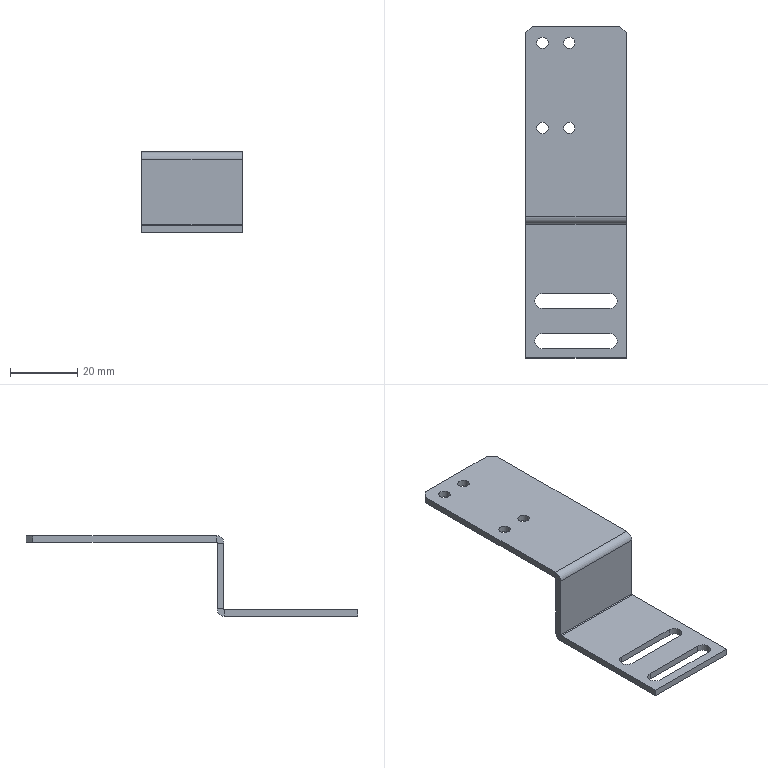Part | NX | 1 solid | 36 faces | box 30 x 99 x 24 mm | volume 6694 mm3 | plane 24 | cylinder 12 | commonest cylinder face diameters 3.4 x4 4.5 x4 0.4 x2 4.4 x2
STEP:
#1=CARTESIAN_POINT('',(30.,-2.,-0.2));
#2=VERTEX_POINT('',#1);
#3=CARTESIAN_POINT('',(30.,-2.,-19.8));
#4=VERTEX_POINT('',#3);
#5=CARTESIAN_POINT('',(30.,-2.,-20.));
#6=DIRECTION('',(0.,0.,-1.));
#7=VECTOR('',#6,1000.);
#8=LINE('',#5,#7);
#9=EDGE_CURVE('',#2,#4,#8,.T.);
#10=ORIENTED_EDGE('',*,*,#9,.T.);
#11=CARTESIAN_POINT('',(30.,0.,-19.8));
#12=VERTEX_POINT('',#11);
#13=CARTESIAN_POINT('',(30.,-2.,-19.8));
#14=DIRECTION('',(0.,1.,0.));
#15=VECTOR('',#14,1000.);
#16=LINE('',#13,#15);
#17=EDGE_CURVE('',#4,#12,#16,.T.);
#18=ORIENTED_EDGE('',*,*,#17,.T.);
#19=CARTESIAN_POINT('',(30.,0.,-0.2));
#20=VERTEX_POINT('',#19);
#21=CARTESIAN_POINT('',(30.,0.,-20.));
#22=DIRECTION('',(0.,0.,-1.));
#23=VECTOR('',#22,1000.);
#24=LINE('',#21,#23);
#25=EDGE_CURVE('',#20,#12,#24,.T.);
#26=ORIENTED_EDGE('',*,*,#25,.F.);
#27=CARTESIAN_POINT('',(30.,0.,-0.2));
#28=DIRECTION('',(0.,-1.,0.));
#29=VECTOR('',#28,1000.);
#30=LINE('',#27,#29);
#31=EDGE_CURVE('',#20,#2,#30,.T.);
#32=ORIENTED_EDGE('',*,*,#31,.T.);
#33=EDGE_LOOP('',(#10,#18,#26,#32));
#34=FACE_BOUND('',#33,.T.);
#35=CARTESIAN_POINT('',(30.,-2.,-20.));
#36=DIRECTION('',(1.,0.,0.));
#37=DIRECTION('',(0.,0.,-1.));
#38=AXIS2_PLACEMENT_3D('',#35,#36,#37);
#39=PLANE('',#38);
#40=ADVANCED_FACE('',(#34),#39,.T.);
#41=CARTESIAN_POINT('',(0.,-2.,-19.8));
#42=VERTEX_POINT('',#41);
#43=CARTESIAN_POINT('',(0.,-2.,-0.2));
#44=VERTEX_POINT('',#43);
#45=CARTESIAN_POINT('',(0.,-2.,0.));
#46=DIRECTION('',(0.,0.,1.));
#47=VECTOR('',#46,1000.);
#48=LINE('',#45,#47);
#49=EDGE_CURVE('',#42,#44,#48,.T.);
#50=ORIENTED_EDGE('',*,*,#49,.F.);
#51=CARTESIAN_POINT('',(30.,-2.,-19.8));
#52=DIRECTION('',(1.,0.,0.));
#53=VECTOR('',#52,1000.);
#54=LINE('',#51,#53);
#55=EDGE_CURVE('',#4,#42,#54,.F.);
#56=ORIENTED_EDGE('',*,*,#55,.F.);
#57=ORIENTED_EDGE('',*,*,#9,.F.);
#58=CARTESIAN_POINT('',(0.,-2.,-0.2));
#59=DIRECTION('',(-1.,0.,0.));
#60=VECTOR('',#59,1000.);
#61=LINE('',#58,#60);
#62=EDGE_CURVE('',#2,#44,#61,.T.);
#63=ORIENTED_EDGE('',*,*,#62,.T.);
#64=EDGE_LOOP('',(#50,#56,#57,#63));
#65=FACE_BOUND('',#64,.T.);
#66=CARTESIAN_POINT('',(0.,-2.,0.));
#67=DIRECTION('',(0.,-1.,0.));
#68=DIRECTION('',(0.,0.,-1.));
#69=AXIS2_PLACEMENT_3D('',#66,#67,#68);
#70=PLANE('',#69);
#71=ADVANCED_FACE('',(#65),#70,.T.);
#72=CARTESIAN_POINT('',(0.,0.,-19.8));
#73=VERTEX_POINT('',#72);
#74=CARTESIAN_POINT('',(30.,0.,-19.8));
#75=DIRECTION('',(1.,0.,0.));
#76=VECTOR('',#75,1000.);
#77=LINE('',#74,#76);
#78=EDGE_CURVE('',#12,#73,#77,.F.);
#79=ORIENTED_EDGE('',*,*,#78,.T.);
#80=CARTESIAN_POINT('',(0.,0.,-0.2));
#81=VERTEX_POINT('',#80);
#82=CARTESIAN_POINT('',(0.,0.,0.));
#83=DIRECTION('',(0.,0.,1.));
#84=VECTOR('',#83,1000.);
#85=LINE('',#82,#84);
#86=EDGE_CURVE('',#73,#81,#85,.T.);
#87=ORIENTED_EDGE('',*,*,#86,.T.);
#88=CARTESIAN_POINT('',(30.,0.,-0.2));
#89=DIRECTION('',(-1.,0.,0.));
#90=VECTOR('',#89,1000.);
#91=LINE('',#88,#90);
#92=EDGE_CURVE('',#20,#81,#91,.T.);
#93=ORIENTED_EDGE('',*,*,#92,.F.);
#94=ORIENTED_EDGE('',*,*,#25,.T.);
#95=EDGE_LOOP('',(#79,#87,#93,#94));
#96=FACE_BOUND('',#95,.T.);
#97=CARTESIAN_POINT('',(0.,0.,0.));
#98=DIRECTION('',(0.,-1.,0.));
#99=DIRECTION('',(0.,0.,-1.));
#100=AXIS2_PLACEMENT_3D('',#97,#98,#99);
#101=PLANE('',#100);
#102=ADVANCED_FACE('',(#96),#101,.F.);
#103=CARTESIAN_POINT('',(14.7,52.,2.));
#104=VERTEX_POINT('',#103);
#105=CARTESIAN_POINT('',(13.,52.,2.));
#106=DIRECTION('',(0.,0.,1.));
#107=DIRECTION('',(1.,0.,0.));
#108=AXIS2_PLACEMENT_3D('',#105,#106,#107);
#109=CIRCLE('',#108,1.7);
#110=EDGE_CURVE('',#104,#104,#109,.T.);
#111=ORIENTED_EDGE('',*,*,#110,.F.);
#112=EDGE_LOOP('',(#111));
#113=FACE_BOUND('',#112,.T.);
#114=CARTESIAN_POINT('',(6.7,52.,2.));
#115=VERTEX_POINT('',#114);
#116=CARTESIAN_POINT('',(5.,52.,2.));
#117=DIRECTION('',(0.,0.,1.));
#118=DIRECTION('',(1.,0.,0.));
#119=AXIS2_PLACEMENT_3D('',#116,#117,#118);
#120=CIRCLE('',#119,1.7);
#121=EDGE_CURVE('',#115,#115,#120,.T.);
#122=ORIENTED_EDGE('',*,*,#121,.F.);
#123=EDGE_LOOP('',(#122));
#124=FACE_BOUND('',#123,.T.);
#125=CARTESIAN_POINT('',(6.7,26.6,2.));
#126=VERTEX_POINT('',#125);
#127=CARTESIAN_POINT('',(5.,26.6,2.));
#128=DIRECTION('',(0.,0.,1.));
#129=DIRECTION('',(1.,0.,0.));
#130=AXIS2_PLACEMENT_3D('',#127,#128,#129);
#131=CIRCLE('',#130,1.7);
#132=EDGE_CURVE('',#126,#126,#131,.T.);
#133=ORIENTED_EDGE('',*,*,#132,.F.);
#134=EDGE_LOOP('',(#133));
#135=FACE_BOUND('',#134,.T.);
#136=CARTESIAN_POINT('',(14.7,26.6,2.));
#137=VERTEX_POINT('',#136);
#138=CARTESIAN_POINT('',(13.,26.6,2.));
#139=DIRECTION('',(0.,0.,1.));
#140=DIRECTION('',(1.,0.,0.));
#141=AXIS2_PLACEMENT_3D('',#138,#139,#140);
#142=CIRCLE('',#141,1.7);
#143=EDGE_CURVE('',#137,#137,#142,.T.);
#144=ORIENTED_EDGE('',*,*,#143,.F.);
#145=EDGE_LOOP('',(#144));
#146=FACE_BOUND('',#145,.T.);
#147=CARTESIAN_POINT('',(2.,57.,2.));
#148=VERTEX_POINT('',#147);
#149=CARTESIAN_POINT('',(28.,57.,2.));
#150=VERTEX_POINT('',#149);
#151=CARTESIAN_POINT('',(0.,57.,2.));
#152=DIRECTION('',(1.,0.,0.));
#153=VECTOR('',#152,1000.);
#154=LINE('',#151,#153);
#155=EDGE_CURVE('',#148,#150,#154,.T.);
#156=ORIENTED_EDGE('',*,*,#155,.F.);
#157=CARTESIAN_POINT('',(0.,55.,2.));
#158=VERTEX_POINT('',#157);
#159=CARTESIAN_POINT('',(0.,55.,2.));
#160=DIRECTION('',(-0.7071,-0.7071,0.));
#161=VECTOR('',#160,1000.);
#162=LINE('',#159,#161);
#163=EDGE_CURVE('',#148,#158,#162,.T.);
#164=ORIENTED_EDGE('',*,*,#163,.T.);
#165=CARTESIAN_POINT('',(0.,0.2,2.));
#166=VERTEX_POINT('',#165);
#167=CARTESIAN_POINT('',(0.,57.,2.));
#168=DIRECTION('',(0.,-1.,0.));
#169=VECTOR('',#168,1000.);
#170=LINE('',#167,#169);
#171=EDGE_CURVE('',#158,#166,#170,.T.);
#172=ORIENTED_EDGE('',*,*,#171,.T.);
#173=CARTESIAN_POINT('',(30.,0.2,2.));
#174=VERTEX_POINT('',#173);
#175=CARTESIAN_POINT('',(0.,0.2,2.));
#176=DIRECTION('',(-1.,0.,0.));
#177=VECTOR('',#176,1000.);
#178=LINE('',#175,#177);
#179=EDGE_CURVE('',#166,#174,#178,.F.);
#180=ORIENTED_EDGE('',*,*,#179,.T.);
#181=CARTESIAN_POINT('',(30.,55.,2.));
#182=VERTEX_POINT('',#181);
#183=CARTESIAN_POINT('',(30.,57.,2.));
#184=DIRECTION('',(0.,-1.,0.));
#185=VECTOR('',#184,1000.);
#186=LINE('',#183,#185);
#187=EDGE_CURVE('',#182,#174,#186,.T.);
#188=ORIENTED_EDGE('',*,*,#187,.F.);
#189=CARTESIAN_POINT('',(30.,55.,2.));
#190=DIRECTION('',(-0.7071,0.7071,0.));
#191=VECTOR('',#190,1000.);
#192=LINE('',#189,#191);
#193=EDGE_CURVE('',#182,#150,#192,.T.);
#194=ORIENTED_EDGE('',*,*,#193,.T.);
#195=EDGE_LOOP('',(#156,#164,#172,#180,#188,#194));
#196=FACE_BOUND('',#195,.T.);
#197=CARTESIAN_POINT('',(0.,57.,2.));
#198=DIRECTION('',(0.,0.,-1.));
#199=DIRECTION('',(-1.,0.,0.));
#200=AXIS2_PLACEMENT_3D('',#197,#198,#199);
#201=PLANE('',#200);
#202=ADVANCED_FACE('',(#113,#124,#135,#146,#196),#201,.F.);
#203=CARTESIAN_POINT('',(11.3,52.,0.));
#204=VERTEX_POINT('',#203);
#205=CARTESIAN_POINT('',(13.,52.,0.));
#206=DIRECTION('',(0.,0.,-1.));
#207=DIRECTION('',(-1.,0.,0.));
#208=AXIS2_PLACEMENT_3D('',#205,#206,#207);
#209=CIRCLE('',#208,1.7);
#210=EDGE_CURVE('',#204,#204,#209,.T.);
#211=ORIENTED_EDGE('',*,*,#210,.F.);
#212=EDGE_LOOP('',(#211));
#213=FACE_BOUND('',#212,.T.);
#214=CARTESIAN_POINT('',(3.3,52.,0.));
#215=VERTEX_POINT('',#214);
#216=CARTESIAN_POINT('',(5.,52.,0.));
#217=DIRECTION('',(0.,0.,-1.));
#218=DIRECTION('',(-1.,0.,0.));
#219=AXIS2_PLACEMENT_3D('',#216,#217,#218);
#220=CIRCLE('',#219,1.7);
#221=EDGE_CURVE('',#215,#215,#220,.T.);
#222=ORIENTED_EDGE('',*,*,#221,.F.);
#223=EDGE_LOOP('',(#222));
#224=FACE_BOUND('',#223,.T.);
#225=CARTESIAN_POINT('',(3.3,26.6,0.));
#226=VERTEX_POINT('',#225);
#227=CARTESIAN_POINT('',(5.,26.6,0.));
#228=DIRECTION('',(0.,0.,-1.));
#229=DIRECTION('',(-1.,0.,0.));
#230=AXIS2_PLACEMENT_3D('',#227,#228,#229);
#231=CIRCLE('',#230,1.7);
#232=EDGE_CURVE('',#226,#226,#231,.T.);
#233=ORIENTED_EDGE('',*,*,#232,.F.);
#234=EDGE_LOOP('',(#233));
#235=FACE_BOUND('',#234,.T.);
#236=CARTESIAN_POINT('',(11.3,26.6,0.));
#237=VERTEX_POINT('',#236);
#238=CARTESIAN_POINT('',(13.,26.6,0.));
#239=DIRECTION('',(0.,0.,-1.));
#240=DIRECTION('',(-1.,0.,0.));
#241=AXIS2_PLACEMENT_3D('',#238,#239,#240);
#242=CIRCLE('',#241,1.7);
#243=EDGE_CURVE('',#237,#237,#242,.T.);
#244=ORIENTED_EDGE('',*,*,#243,.F.);
#245=EDGE_LOOP('',(#244));
#246=FACE_BOUND('',#245,.T.);
#247=CARTESIAN_POINT('',(0.,55.,0.));
#248=VERTEX_POINT('',#247);
#249=CARTESIAN_POINT('',(0.,0.2,0.));
#250=VERTEX_POINT('',#249);
#251=CARTESIAN_POINT('',(0.,57.,0.));
#252=DIRECTION('',(0.,-1.,0.));
#253=VECTOR('',#252,1000.);
#254=LINE('',#251,#253);
#255=EDGE_CURVE('',#248,#250,#254,.T.);
#256=ORIENTED_EDGE('',*,*,#255,.F.);
#257=CARTESIAN_POINT('',(2.,57.,0.));
#258=VERTEX_POINT('',#257);
#259=CARTESIAN_POINT('',(1.,56.,0.));
#260=DIRECTION('',(0.7071,0.7071,0.));
#261=VECTOR('',#260,1000.);
#262=LINE('',#259,#261);
#263=EDGE_CURVE('',#248,#258,#262,.T.);
#264=ORIENTED_EDGE('',*,*,#263,.T.);
#265=CARTESIAN_POINT('',(28.,57.,0.));
#266=VERTEX_POINT('',#265);
#267=CARTESIAN_POINT('',(0.,57.,0.));
#268=DIRECTION('',(1.,0.,0.));
#269=VECTOR('',#268,1000.);
#270=LINE('',#267,#269);
#271=EDGE_CURVE('',#258,#266,#270,.T.);
#272=ORIENTED_EDGE('',*,*,#271,.T.);
#273=CARTESIAN_POINT('',(30.,55.,0.));
#274=VERTEX_POINT('',#273);
#275=CARTESIAN_POINT('',(14.,71.,0.));
#276=DIRECTION('',(0.7071,-0.7071,0.));
#277=VECTOR('',#276,1000.);
#278=LINE('',#275,#277);
#279=EDGE_CURVE('',#266,#274,#278,.T.);
#280=ORIENTED_EDGE('',*,*,#279,.T.);
#281=CARTESIAN_POINT('',(30.,0.2,0.));
#282=VERTEX_POINT('',#281);
#283=CARTESIAN_POINT('',(30.,57.,0.));
#284=DIRECTION('',(0.,-1.,0.));
#285=VECTOR('',#284,1000.);
#286=LINE('',#283,#285);
#287=EDGE_CURVE('',#274,#282,#286,.T.);
#288=ORIENTED_EDGE('',*,*,#287,.T.);
#289=CARTESIAN_POINT('',(0.,0.2,0.));
#290=DIRECTION('',(-1.,0.,0.));
#291=VECTOR('',#290,1000.);
#292=LINE('',#289,#291);
#293=EDGE_CURVE('',#250,#282,#292,.F.);
#294=ORIENTED_EDGE('',*,*,#293,.F.);
#295=EDGE_LOOP('',(#256,#264,#272,#280,#288,#294));
#296=FACE_BOUND('',#295,.T.);
#297=CARTESIAN_POINT('',(0.,57.,0.));
#298=DIRECTION('',(0.,0.,-1.));
#299=DIRECTION('',(-1.,0.,0.));
#300=AXIS2_PLACEMENT_3D('',#297,#298,#299);
#301=PLANE('',#300);
#302=ADVANCED_FACE('',(#213,#224,#235,#246,#296),#301,.T.);
#303=ORIENTED_EDGE('',*,*,#171,.F.);
#304=CARTESIAN_POINT('',(0.,55.,0.));
#305=DIRECTION('',(0.,0.,-1.));
#306=VECTOR('',#305,1000.);
#307=LINE('',#304,#306);
#308=EDGE_CURVE('',#158,#248,#307,.T.);
#309=ORIENTED_EDGE('',*,*,#308,.T.);
#310=ORIENTED_EDGE('',*,*,#255,.T.);
#311=CARTESIAN_POINT('',(0.,0.2,0.));
#312=DIRECTION('',(0.,0.,1.));
#313=VECTOR('',#312,1000.);
#314=LINE('',#311,#313);
#315=EDGE_CURVE('',#250,#166,#314,.T.);
#316=ORIENTED_EDGE('',*,*,#315,.T.);
#317=EDGE_LOOP('',(#303,#309,#310,#316));
#318=FACE_BOUND('',#317,.T.);
#319=CARTESIAN_POINT('',(0.,57.,2.));
#320=DIRECTION('',(-1.,0.,0.));
#321=DIRECTION('',(0.,0.,1.));
#322=AXIS2_PLACEMENT_3D('',#319,#320,#321);
#323=PLANE('',#322);
#324=ADVANCED_FACE('',(#318),#323,.T.);
#325=ORIENTED_EDGE('',*,*,#287,.F.);
#326=CARTESIAN_POINT('',(30.,55.,2.));
#327=DIRECTION('',(0.,0.,1.));
#328=VECTOR('',#327,1000.);
#329=LINE('',#326,#328);
#330=EDGE_CURVE('',#274,#182,#329,.T.);
#331=ORIENTED_EDGE('',*,*,#330,.T.);
#332=ORIENTED_EDGE('',*,*,#187,.T.);
#333=CARTESIAN_POINT('',(30.,0.2,0.));
#334=DIRECTION('',(0.,0.,1.));
#335=VECTOR('',#334,1000.);
#336=LINE('',#333,#335);
#337=EDGE_CURVE('',#282,#174,#336,.T.);
#338=ORIENTED_EDGE('',*,*,#337,.F.);
#339=EDGE_LOOP('',(#325,#331,#332,#338));
#340=FACE_BOUND('',#339,.T.);
#341=CARTESIAN_POINT('',(30.,57.,0.));
#342=DIRECTION('',(1.,0.,0.));
#343=DIRECTION('',(0.,0.,-1.));
#344=AXIS2_PLACEMENT_3D('',#341,#342,#343);
#345=PLANE('',#344);
#346=ADVANCED_FACE('',(#340),#345,.T.);
#347=ORIENTED_EDGE('',*,*,#271,.F.);
#348=CARTESIAN_POINT('',(2.,57.,2.));
#349=DIRECTION('',(0.,0.,1.));
#350=VECTOR('',#349,1000.);
#351=LINE('',#348,#350);
#352=EDGE_CURVE('',#258,#148,#351,.T.);
#353=ORIENTED_EDGE('',*,*,#352,.T.);
#354=ORIENTED_EDGE('',*,*,#155,.T.);
#355=CARTESIAN_POINT('',(28.,57.,0.));
#356=DIRECTION('',(0.,0.,-1.));
#357=VECTOR('',#356,1000.);
#358=LINE('',#355,#357);
#359=EDGE_CURVE('',#150,#266,#358,.T.);
#360=ORIENTED_EDGE('',*,*,#359,.T.);
#361=EDGE_LOOP('',(#347,#353,#354,#360));
#362=FACE_BOUND('',#361,.T.);
#363=CARTESIAN_POINT('',(0.,57.,0.));
#364=DIRECTION('',(0.,-1.,0.));
#365=DIRECTION('',(-1.,0.,0.));
#366=AXIS2_PLACEMENT_3D('',#363,#364,#365);
#367=PLANE('',#366);
#368=ADVANCED_FACE('',(#362),#367,.F.);
#369=ORIENTED_EDGE('',*,*,#31,.F.);
#370=CARTESIAN_POINT('',(30.,0.2,-0.2));
#371=DIRECTION('',(-1.,0.,0.));
#372=DIRECTION('',(0.,-1.,0.));
#373=AXIS2_PLACEMENT_3D('',#370,#371,#372);
#374=CIRCLE('',#373,0.2);
#375=EDGE_CURVE('',#282,#20,#374,.F.);
#376=ORIENTED_EDGE('',*,*,#375,.F.);
#377=ORIENTED_EDGE('',*,*,#337,.T.);
#378=CARTESIAN_POINT('',(30.,0.2,-0.2));
#379=DIRECTION('',(-1.,0.,0.));
#380=DIRECTION('',(0.,-1.,0.));
#381=AXIS2_PLACEMENT_3D('',#378,#379,#380);
#382=CIRCLE('',#381,2.2);
#383=EDGE_CURVE('',#174,#2,#382,.F.);
#384=ORIENTED_EDGE('',*,*,#383,.T.);
#385=EDGE_LOOP('',(#369,#376,#377,#384));
#386=FACE_BOUND('',#385,.T.);
#387=CARTESIAN_POINT('',(30.,0.2,-0.2));
#388=DIRECTION('',(1.,0.,0.));
#389=DIRECTION('',(0.,1.,0.));
#390=AXIS2_PLACEMENT_3D('',#387,#388,#389);
#391=PLANE('',#390);
#392=ADVANCED_FACE('',(#386),#391,.T.);
#393=CARTESIAN_POINT('',(0.,0.2,-0.2));
#394=DIRECTION('',(-1.,0.,0.));
#395=DIRECTION('',(0.,-1.,0.));
#396=AXIS2_PLACEMENT_3D('',#393,#394,#395);
#397=CIRCLE('',#396,0.2);
#398=EDGE_CURVE('',#81,#250,#397,.T.);
#399=ORIENTED_EDGE('',*,*,#398,.F.);
#400=CARTESIAN_POINT('',(0.,0.,-0.2));
#401=DIRECTION('',(0.,-1.,0.));
#402=VECTOR('',#401,1000.);
#403=LINE('',#400,#402);
#404=EDGE_CURVE('',#81,#44,#403,.T.);
#405=ORIENTED_EDGE('',*,*,#404,.T.);
#406=CARTESIAN_POINT('',(0.,0.2,-0.2));
#407=DIRECTION('',(-1.,0.,0.));
#408=DIRECTION('',(0.,-1.,0.));
#409=AXIS2_PLACEMENT_3D('',#406,#407,#408);
#410=CIRCLE('',#409,2.2);
#411=EDGE_CURVE('',#44,#166,#410,.T.);
#412=ORIENTED_EDGE('',*,*,#411,.T.);
#413=ORIENTED_EDGE('',*,*,#315,.F.);
#414=EDGE_LOOP('',(#399,#405,#412,#413));
#415=FACE_BOUND('',#414,.T.);
#416=CARTESIAN_POINT('',(0.,0.2,-0.2));
#417=DIRECTION('',(1.,0.,0.));
#418=DIRECTION('',(0.,1.,0.));
#419=AXIS2_PLACEMENT_3D('',#416,#417,#418);
#420=PLANE('',#419);
#421=ADVANCED_FACE('',(#415),#420,.F.);
#422=ORIENTED_EDGE('',*,*,#179,.F.);
#423=ORIENTED_EDGE('',*,*,#411,.F.);
#424=ORIENTED_EDGE('',*,*,#62,.F.);
#425=ORIENTED_EDGE('',*,*,#383,.F.);
#426=EDGE_LOOP('',(#422,#423,#424,#425));
#427=FACE_BOUND('',#426,.T.);
#428=CARTESIAN_POINT('',(0.,0.2,-0.2));
#429=DIRECTION('',(-1.,0.,0.));
#430=DIRECTION('',(0.,-1.,0.));
#431=AXIS2_PLACEMENT_3D('',#428,#429,#430);
#432=CYLINDRICAL_SURFACE('',#431,2.2);
#433=ADVANCED_FACE('',(#427),#432,.T.);
#434=ORIENTED_EDGE('',*,*,#293,.T.);
#435=ORIENTED_EDGE('',*,*,#375,.T.);
#436=ORIENTED_EDGE('',*,*,#92,.T.);
#437=ORIENTED_EDGE('',*,*,#398,.T.);
#438=EDGE_LOOP('',(#434,#435,#436,#437));
#439=FACE_BOUND('',#438,.T.);
#440=CARTESIAN_POINT('',(0.,0.2,-0.2));
#441=DIRECTION('',(-1.,0.,0.));
#442=DIRECTION('',(0.,-1.,0.));
#443=AXIS2_PLACEMENT_3D('',#440,#441,#442);
#444=CYLINDRICAL_SURFACE('',#443,0.2);
#445=ADVANCED_FACE('',(#439),#444,.F.);
#446=CARTESIAN_POINT('',(0.,-2.,-19.8));
#447=DIRECTION('',(0.,1.,0.));
#448=VECTOR('',#447,1000.);
#449=LINE('',#446,#448);
#450=EDGE_CURVE('',#42,#73,#449,.T.);
#451=ORIENTED_EDGE('',*,*,#450,.F.);
#452=ORIENTED_EDGE('',*,*,#49,.T.);
#453=ORIENTED_EDGE('',*,*,#404,.F.);
#454=ORIENTED_EDGE('',*,*,#86,.F.);
#455=EDGE_LOOP('',(#451,#452,#453,#454));
#456=FACE_BOUND('',#455,.T.);
#457=CARTESIAN_POINT('',(0.,-2.,0.));
#458=DIRECTION('',(-1.,0.,0.));
#459=DIRECTION('',(0.,0.,1.));
#460=AXIS2_PLACEMENT_3D('',#457,#458,#459);
#461=PLANE('',#460);
#462=ADVANCED_FACE('',(#456),#461,.T.);
#463=ORIENTED_EDGE('',*,*,#243,.T.);
#464=EDGE_LOOP('',(#463));
#465=FACE_BOUND('',#464,.T.);
#466=ORIENTED_EDGE('',*,*,#143,.T.);
#467=EDGE_LOOP('',(#466));
#468=FACE_BOUND('',#467,.T.);
#469=CARTESIAN_POINT('',(13.,26.6,2.));
#470=DIRECTION('',(0.,0.,1.));
#471=DIRECTION('',(1.,0.,0.));
#472=AXIS2_PLACEMENT_3D('',#469,#470,#471);
#473=CYLINDRICAL_SURFACE('',#472,1.7);
#474=ADVANCED_FACE('',(#465,#468),#473,.F.);
#475=ORIENTED_EDGE('',*,*,#232,.T.);
#476=EDGE_LOOP('',(#475));
#477=FACE_BOUND('',#476,.T.);
#478=ORIENTED_EDGE('',*,*,#132,.T.);
#479=EDGE_LOOP('',(#478));
#480=FACE_BOUND('',#479,.T.);
#481=CARTESIAN_POINT('',(5.,26.6,2.));
#482=DIRECTION('',(0.,0.,1.));
#483=DIRECTION('',(1.,0.,0.));
#484=AXIS2_PLACEMENT_3D('',#481,#482,#483);
#485=CYLINDRICAL_SURFACE('',#484,1.7);
#486=ADVANCED_FACE('',(#477,#480),#485,.F.);
#487=ORIENTED_EDGE('',*,*,#221,.T.);
#488=EDGE_LOOP('',(#487));
#489=FACE_BOUND('',#488,.T.);
#490=ORIENTED_EDGE('',*,*,#121,.T.);
#491=EDGE_LOOP('',(#490));
#492=FACE_BOUND('',#491,.T.);
#493=CARTESIAN_POINT('',(5.,52.,2.));
#494=DIRECTION('',(0.,0.,1.));
#495=DIRECTION('',(1.,0.,0.));
#496=AXIS2_PLACEMENT_3D('',#493,#494,#495);
#497=CYLINDRICAL_SURFACE('',#496,1.7);
#498=ADVANCED_FACE('',(#489,#492),#497,.F.);
#499=ORIENTED_EDGE('',*,*,#210,.T.);
#500=EDGE_LOOP('',(#499));
#501=FACE_BOUND('',#500,.T.);
#502=ORIENTED_EDGE('',*,*,#110,.T.);
#503=EDGE_LOOP('',(#502));
#504=FACE_BOUND('',#503,.T.);
#505=CARTESIAN_POINT('',(13.,52.,2.));
#506=DIRECTION('',(0.,0.,1.));
#507=DIRECTION('',(1.,0.,0.));
#508=AXIS2_PLACEMENT_3D('',#505,#506,#507);
#509=CYLINDRICAL_SURFACE('',#508,1.7);
#510=ADVANCED_FACE('',(#501,#504),#509,.F.);
#511=CARTESIAN_POINT('',(0.,-2.2,-20.));
#512=VERTEX_POINT('',#511);
#513=CARTESIAN_POINT('',(0.,-2.2,-22.));
#514=VERTEX_POINT('',#513);
#515=CARTESIAN_POINT('',(0.,-2.2,-20.));
#516=DIRECTION('',(0.,0.,-1.));
#517=VECTOR('',#516,1000.);
#518=LINE('',#515,#517);
#519=EDGE_CURVE('',#512,#514,#518,.T.);
#520=ORIENTED_EDGE('',*,*,#519,.F.);
#521=CARTESIAN_POINT('',(0.,-2.2,-19.8));
#522=DIRECTION('',(1.,0.,0.));
#523=DIRECTION('',(0.,0.,-1.));
#524=AXIS2_PLACEMENT_3D('',#521,#522,#523);
#525=CIRCLE('',#524,0.2);
#526=EDGE_CURVE('',#42,#512,#525,.F.);
#527=ORIENTED_EDGE('',*,*,#526,.F.);
#528=ORIENTED_EDGE('',*,*,#450,.T.);
#529=CARTESIAN_POINT('',(0.,-2.2,-19.8));
#530=DIRECTION('',(1.,0.,0.));
#531=DIRECTION('',(0.,0.,-1.));
#532=AXIS2_PLACEMENT_3D('',#529,#530,#531);
#533=CIRCLE('',#532,2.2);
#534=EDGE_CURVE('',#73,#514,#533,.F.);
#535=ORIENTED_EDGE('',*,*,#534,.T.);
#536=EDGE_LOOP('',(#520,#527,#528,#535));
#537=FACE_BOUND('',#536,.T.);
#538=CARTESIAN_POINT('',(0.,-2.2,-19.8));
#539=DIRECTION('',(-1.,0.,0.));
#540=DIRECTION('',(0.,0.,1.));
#541=AXIS2_PLACEMENT_3D('',#538,#539,#540);
#542=PLANE('',#541);
#543=ADVANCED_FACE('',(#537),#542,.T.);
#544=CARTESIAN_POINT('',(30.,-2.2,-20.));
#545=VERTEX_POINT('',#544);
#546=CARTESIAN_POINT('',(30.,-2.2,-19.8));
#547=DIRECTION('',(1.,0.,0.));
#548=DIRECTION('',(0.,0.,-1.));
#549=AXIS2_PLACEMENT_3D('',#546,#547,#548);
#550=CIRCLE('',#549,0.2);
#551=EDGE_CURVE('',#545,#4,#550,.T.);
#552=ORIENTED_EDGE('',*,*,#551,.F.);
#553=CARTESIAN_POINT('',(30.,-2.2,-22.));
#554=VERTEX_POINT('',#553);
#555=CARTESIAN_POINT('',(30.,-2.2,-20.));
#556=DIRECTION('',(0.,0.,-1.));
#557=VECTOR('',#556,1000.);
#558=LINE('',#555,#557);
#559=EDGE_CURVE('',#545,#554,#558,.T.);
#560=ORIENTED_EDGE('',*,*,#559,.T.);
#561=CARTESIAN_POINT('',(30.,-2.2,-19.8));
#562=DIRECTION('',(1.,0.,0.));
#563=DIRECTION('',(0.,0.,-1.));
#564=AXIS2_PLACEMENT_3D('',#561,#562,#563);
#565=CIRCLE('',#564,2.2);
#566=EDGE_CURVE('',#554,#12,#565,.T.);
#567=ORIENTED_EDGE('',*,*,#566,.T.);
#568=ORIENTED_EDGE('',*,*,#17,.F.);
#569=EDGE_LOOP('',(#552,#560,#567,#568));
#570=FACE_BOUND('',#569,.T.);
#571=CARTESIAN_POINT('',(30.,-2.2,-19.8));
#572=DIRECTION('',(-1.,0.,0.));
#573=DIRECTION('',(0.,0.,1.));
#574=AXIS2_PLACEMENT_3D('',#571,#572,#573);
#575=PLANE('',#574);
#576=ADVANCED_FACE('',(#570),#575,.F.);
#577=ORIENTED_EDGE('',*,*,#78,.F.);
#578=ORIENTED_EDGE('',*,*,#566,.F.);
#579=CARTESIAN_POINT('',(0.,-2.2,-22.));
#580=DIRECTION('',(-1.,0.,0.));
#581=VECTOR('',#580,1000.);
#582=LINE('',#579,#581);
#583=EDGE_CURVE('',#554,#514,#582,.T.);
#584=ORIENTED_EDGE('',*,*,#583,.T.);
#585=ORIENTED_EDGE('',*,*,#534,.F.);
#586=EDGE_LOOP('',(#577,#578,#584,#585));
#587=FACE_BOUND('',#586,.T.);
#588=CARTESIAN_POINT('',(30.,-2.2,-19.8));
#589=DIRECTION('',(1.,0.,0.));
#590=DIRECTION('',(0.,0.,-1.));
#591=AXIS2_PLACEMENT_3D('',#588,#589,#590);
#592=CYLINDRICAL_SURFACE('',#591,2.2);
#593=ADVANCED_FACE('',(#587),#592,.T.);
#594=ORIENTED_EDGE('',*,*,#55,.T.);
#595=ORIENTED_EDGE('',*,*,#526,.T.);
#596=CARTESIAN_POINT('',(0.,-2.2,-20.));
#597=DIRECTION('',(1.,0.,0.));
#598=VECTOR('',#597,1000.);
#599=LINE('',#596,#598);
#600=EDGE_CURVE('',#512,#545,#599,.T.);
#601=ORIENTED_EDGE('',*,*,#600,.T.);
#602=ORIENTED_EDGE('',*,*,#551,.T.);
#603=EDGE_LOOP('',(#594,#595,#601,#602));
#604=FACE_BOUND('',#603,.T.);
#605=CARTESIAN_POINT('',(30.,-2.2,-19.8));
#606=DIRECTION('',(1.,0.,0.));
#607=DIRECTION('',(0.,0.,-1.));
#608=AXIS2_PLACEMENT_3D('',#605,#606,#607);
#609=CYLINDRICAL_SURFACE('',#608,0.2);
#610=ADVANCED_FACE('',(#604),#609,.F.);
#611=ORIENTED_EDGE('',*,*,#559,.F.);
#612=CARTESIAN_POINT('',(30.,-42.,-20.));
#613=VERTEX_POINT('',#612);
#614=CARTESIAN_POINT('',(30.,-42.,-20.));
#615=DIRECTION('',(0.,-1.,0.));
#616=VECTOR('',#615,1000.);
#617=LINE('',#614,#616);
#618=EDGE_CURVE('',#545,#613,#617,.T.);
#619=ORIENTED_EDGE('',*,*,#618,.T.);
#620=CARTESIAN_POINT('',(30.,-42.,-22.));
#621=VERTEX_POINT('',#620);
#622=CARTESIAN_POINT('',(30.,-42.,-22.));
#623=DIRECTION('',(0.,0.,1.));
#624=VECTOR('',#623,1000.);
#625=LINE('',#622,#624);
#626=EDGE_CURVE('',#621,#613,#625,.T.);
#627=ORIENTED_EDGE('',*,*,#626,.F.);
#628=CARTESIAN_POINT('',(30.,-42.,-22.));
#629=DIRECTION('',(0.,-1.,0.));
#630=VECTOR('',#629,1000.);
#631=LINE('',#628,#630);
#632=EDGE_CURVE('',#554,#621,#631,.T.);
#633=ORIENTED_EDGE('',*,*,#632,.F.);
#634=EDGE_LOOP('',(#611,#619,#627,#633));
#635=FACE_BOUND('',#634,.T.);
#636=CARTESIAN_POINT('',(30.,-42.,-22.));
#637=DIRECTION('',(-1.,0.,0.));
#638=DIRECTION('',(0.,0.,1.));
#639=AXIS2_PLACEMENT_3D('',#636,#637,#638);
#640=PLANE('',#639);
#641=ADVANCED_FACE('',(#635),#640,.F.);
#642=ORIENTED_EDGE('',*,*,#519,.T.);
#643=CARTESIAN_POINT('',(0.,-42.,-22.));
#644=VERTEX_POINT('',#643);
#645=CARTESIAN_POINT('',(0.,-2.,-22.));
#646=DIRECTION('',(0.,1.,0.));
#647=VECTOR('',#646,1000.);
#648=LINE('',#645,#647);
#649=EDGE_CURVE('',#644,#514,#648,.T.);
#650=ORIENTED_EDGE('',*,*,#649,.F.);
#651=CARTESIAN_POINT('',(0.,-42.,-20.));
#652=VERTEX_POINT('',#651);
#653=CARTESIAN_POINT('',(0.,-42.,-22.));
#654=DIRECTION('',(0.,0.,1.));
#655=VECTOR('',#654,1000.);
#656=LINE('',#653,#655);
#657=EDGE_CURVE('',#644,#652,#656,.T.);
#658=ORIENTED_EDGE('',*,*,#657,.T.);
#659=CARTESIAN_POINT('',(0.,-2.,-20.));
#660=DIRECTION('',(0.,1.,0.));
#661=VECTOR('',#660,1000.);
#662=LINE('',#659,#661);
#663=EDGE_CURVE('',#652,#512,#662,.T.);
#664=ORIENTED_EDGE('',*,*,#663,.T.);
#665=EDGE_LOOP('',(#642,#650,#658,#664));
#666=FACE_BOUND('',#665,.T.);
#667=CARTESIAN_POINT('',(0.,-2.,-22.));
#668=DIRECTION('',(1.,0.,0.));
#669=DIRECTION('',(0.,0.,-1.));
#670=AXIS2_PLACEMENT_3D('',#667,#668,#669);
#671=PLANE('',#670);
#672=ADVANCED_FACE('',(#666),#671,.F.);
#673=CARTESIAN_POINT('',(25.,-34.75,-22.));
#674=VERTEX_POINT('',#673);
#675=CARTESIAN_POINT('',(5.,-34.75,-22.));
#676=VERTEX_POINT('',#675);
#677=CARTESIAN_POINT('',(0.,-34.75,-22.));
#678=DIRECTION('',(-1.,0.,0.));
#679=VECTOR('',#678,1000.);
#680=LINE('',#677,#679);
#681=EDGE_CURVE('',#674,#676,#680,.T.);
#682=ORIENTED_EDGE('',*,*,#681,.T.);
#683=CARTESIAN_POINT('',(5.,-39.25,-22.));
#684=VERTEX_POINT('',#683);
#685=CARTESIAN_POINT('',(5.,-37.,-22.));
#686=DIRECTION('',(0.,0.,1.));
#687=DIRECTION('',(1.,0.,0.));
#688=AXIS2_PLACEMENT_3D('',#685,#686,#687);
#689=CIRCLE('',#688,2.25);
#690=EDGE_CURVE('',#676,#684,#689,.T.);
#691=ORIENTED_EDGE('',*,*,#690,.T.);
#692=CARTESIAN_POINT('',(25.,-39.25,-22.));
#693=VERTEX_POINT('',#692);
#694=CARTESIAN_POINT('',(0.,-39.25,-22.));
#695=DIRECTION('',(1.,0.,0.));
#696=VECTOR('',#695,1000.);
#697=LINE('',#694,#696);
#698=EDGE_CURVE('',#684,#693,#697,.T.);
#699=ORIENTED_EDGE('',*,*,#698,.T.);
#700=CARTESIAN_POINT('',(25.,-37.,-22.));
#701=DIRECTION('',(0.,0.,1.));
#702=DIRECTION('',(1.,0.,0.));
#703=AXIS2_PLACEMENT_3D('',#700,#701,#702);
#704=CIRCLE('',#703,2.25);
#705=EDGE_CURVE('',#693,#674,#704,.T.);
#706=ORIENTED_EDGE('',*,*,#705,.T.);
#707=EDGE_LOOP('',(#682,#691,#699,#706));
#708=FACE_BOUND('',#707,.T.);
#709=CARTESIAN_POINT('',(25.,-22.75,-22.));
#710=VERTEX_POINT('',#709);
#711=CARTESIAN_POINT('',(5.,-22.75,-22.));
#712=VERTEX_POINT('',#711);
#713=CARTESIAN_POINT('',(0.,-22.75,-22.));
#714=DIRECTION('',(-1.,0.,0.));
#715=VECTOR('',#714,1000.);
#716=LINE('',#713,#715);
#717=EDGE_CURVE('',#710,#712,#716,.T.);
#718=ORIENTED_EDGE('',*,*,#717,.T.);
#719=CARTESIAN_POINT('',(5.,-27.25,-22.));
#720=VERTEX_POINT('',#719);
#721=CARTESIAN_POINT('',(5.,-25.,-22.));
#722=DIRECTION('',(0.,0.,1.));
#723=DIRECTION('',(1.,0.,0.));
#724=AXIS2_PLACEMENT_3D('',#721,#722,#723);
#725=CIRCLE('',#724,2.25);
#726=EDGE_CURVE('',#712,#720,#725,.T.);
#727=ORIENTED_EDGE('',*,*,#726,.T.);
#728=CARTESIAN_POINT('',(25.,-27.25,-22.));
#729=VERTEX_POINT('',#728);
#730=CARTESIAN_POINT('',(0.,-27.25,-22.));
#731=DIRECTION('',(1.,0.,0.));
#732=VECTOR('',#731,1000.);
#733=LINE('',#730,#732);
#734=EDGE_CURVE('',#720,#729,#733,.T.);
#735=ORIENTED_EDGE('',*,*,#734,.T.);
#736=CARTESIAN_POINT('',(25.,-25.,-22.));
#737=DIRECTION('',(0.,0.,1.));
#738=DIRECTION('',(1.,0.,0.));
#739=AXIS2_PLACEMENT_3D('',#736,#737,#738);
#740=CIRCLE('',#739,2.25);
#741=EDGE_CURVE('',#729,#710,#740,.T.);
#742=ORIENTED_EDGE('',*,*,#741,.T.);
#743=EDGE_LOOP('',(#718,#727,#735,#742));
#744=FACE_BOUND('',#743,.T.);
#745=ORIENTED_EDGE('',*,*,#583,.F.);
#746=ORIENTED_EDGE('',*,*,#632,.T.);
#747=CARTESIAN_POINT('',(0.,-42.,-22.));
#748=DIRECTION('',(-1.,0.,0.));
#749=VECTOR('',#748,1000.);
#750=LINE('',#747,#749);
#751=EDGE_CURVE('',#621,#644,#750,.T.);
#752=ORIENTED_EDGE('',*,*,#751,.T.);
#753=ORIENTED_EDGE('',*,*,#649,.T.);
#754=EDGE_LOOP('',(#745,#746,#752,#753));
#755=FACE_BOUND('',#754,.T.);
#756=CARTESIAN_POINT('',(0.,0.,-22.));
#757=DIRECTION('',(0.,0.,1.));
#758=DIRECTION('',(1.,0.,0.));
#759=AXIS2_PLACEMENT_3D('',#756,#757,#758);
#760=PLANE('',#759);
#761=ADVANCED_FACE('',(#708,#744,#755),#760,.F.);
#762=CARTESIAN_POINT('',(5.,-34.75,-20.));
#763=VERTEX_POINT('',#762);
#764=CARTESIAN_POINT('',(5.,-39.25,-20.));
#765=VERTEX_POINT('',#764);
#766=CARTESIAN_POINT('',(5.,-37.,-20.));
#767=DIRECTION('',(0.,0.,1.));
#768=DIRECTION('',(1.,0.,0.));
#769=AXIS2_PLACEMENT_3D('',#766,#767,#768);
#770=CIRCLE('',#769,2.25);
#771=EDGE_CURVE('',#763,#765,#770,.T.);
#772=ORIENTED_EDGE('',*,*,#771,.F.);
#773=CARTESIAN_POINT('',(25.,-34.75,-20.));
#774=VERTEX_POINT('',#773);
#775=CARTESIAN_POINT('',(5.,-34.75,-20.));
#776=DIRECTION('',(-1.,0.,0.));
#777=VECTOR('',#776,1000.);
#778=LINE('',#775,#777);
#779=EDGE_CURVE('',#774,#763,#778,.T.);
#780=ORIENTED_EDGE('',*,*,#779,.F.);
#781=CARTESIAN_POINT('',(25.,-39.25,-20.));
#782=VERTEX_POINT('',#781);
#783=CARTESIAN_POINT('',(25.,-37.,-20.));
#784=DIRECTION('',(0.,0.,1.));
#785=DIRECTION('',(1.,0.,0.));
#786=AXIS2_PLACEMENT_3D('',#783,#784,#785);
#787=CIRCLE('',#786,2.25);
#788=EDGE_CURVE('',#782,#774,#787,.T.);
#789=ORIENTED_EDGE('',*,*,#788,.F.);
#790=CARTESIAN_POINT('',(5.,-39.25,-20.));
#791=DIRECTION('',(1.,0.,0.));
#792=VECTOR('',#791,1000.);
#793=LINE('',#790,#792);
#794=EDGE_CURVE('',#765,#782,#793,.T.);
#795=ORIENTED_EDGE('',*,*,#794,.F.);
#796=EDGE_LOOP('',(#772,#780,#789,#795));
#797=FACE_BOUND('',#796,.T.);
#798=CARTESIAN_POINT('',(5.,-22.75,-20.));
#799=VERTEX_POINT('',#798);
#800=CARTESIAN_POINT('',(5.,-27.25,-20.));
#801=VERTEX_POINT('',#800);
#802=CARTESIAN_POINT('',(5.,-25.,-20.));
#803=DIRECTION('',(0.,0.,1.));
#804=DIRECTION('',(1.,0.,0.));
#805=AXIS2_PLACEMENT_3D('',#802,#803,#804);
#806=CIRCLE('',#805,2.25);
#807=EDGE_CURVE('',#799,#801,#806,.T.);
#808=ORIENTED_EDGE('',*,*,#807,.F.);
#809=CARTESIAN_POINT('',(25.,-22.75,-20.));
#810=VERTEX_POINT('',#809);
#811=CARTESIAN_POINT('',(5.,-22.75,-20.));
#812=DIRECTION('',(-1.,0.,0.));
#813=VECTOR('',#812,1000.);
#814=LINE('',#811,#813);
#815=EDGE_CURVE('',#810,#799,#814,.T.);
#816=ORIENTED_EDGE('',*,*,#815,.F.);
#817=CARTESIAN_POINT('',(25.,-27.25,-20.));
#818=VERTEX_POINT('',#817);
#819=CARTESIAN_POINT('',(25.,-25.,-20.));
#820=DIRECTION('',(0.,0.,1.));
#821=DIRECTION('',(1.,0.,0.));
#822=AXIS2_PLACEMENT_3D('',#819,#820,#821);
#823=CIRCLE('',#822,2.25);
#824=EDGE_CURVE('',#818,#810,#823,.T.);
#825=ORIENTED_EDGE('',*,*,#824,.F.);
#826=CARTESIAN_POINT('',(5.,-27.25,-20.));
#827=DIRECTION('',(1.,0.,0.));
#828=VECTOR('',#827,1000.);
#829=LINE('',#826,#828);
#830=EDGE_CURVE('',#801,#818,#829,.T.);
#831=ORIENTED_EDGE('',*,*,#830,.F.);
#832=EDGE_LOOP('',(#808,#816,#825,#831));
#833=FACE_BOUND('',#832,.T.);
#834=ORIENTED_EDGE('',*,*,#618,.F.);
#835=ORIENTED_EDGE('',*,*,#600,.F.);
#836=ORIENTED_EDGE('',*,*,#663,.F.);
#837=CARTESIAN_POINT('',(0.,-42.,-20.));
#838=DIRECTION('',(-1.,0.,0.));
#839=VECTOR('',#838,1000.);
#840=LINE('',#837,#839);
#841=EDGE_CURVE('',#613,#652,#840,.T.);
#842=ORIENTED_EDGE('',*,*,#841,.F.);
#843=EDGE_LOOP('',(#834,#835,#836,#842));
#844=FACE_BOUND('',#843,.T.);
#845=CARTESIAN_POINT('',(0.,0.,-20.));
#846=DIRECTION('',(0.,0.,1.));
#847=DIRECTION('',(1.,0.,0.));
#848=AXIS2_PLACEMENT_3D('',#845,#846,#847);
#849=PLANE('',#848);
#850=ADVANCED_FACE('',(#797,#833,#844),#849,.T.);
#851=ORIENTED_EDGE('',*,*,#841,.T.);
#852=ORIENTED_EDGE('',*,*,#657,.F.);
#853=ORIENTED_EDGE('',*,*,#751,.F.);
#854=ORIENTED_EDGE('',*,*,#626,.T.);
#855=EDGE_LOOP('',(#851,#852,#853,#854));
#856=FACE_BOUND('',#855,.T.);
#857=CARTESIAN_POINT('',(0.,-42.,-22.));
#858=DIRECTION('',(0.,1.,0.));
#859=DIRECTION('',(0.,0.,1.));
#860=AXIS2_PLACEMENT_3D('',#857,#858,#859);
#861=PLANE('',#860);
#862=ADVANCED_FACE('',(#856),#861,.F.);
#863=ORIENTED_EDGE('',*,*,#163,.F.);
#864=ORIENTED_EDGE('',*,*,#352,.F.);
#865=ORIENTED_EDGE('',*,*,#263,.F.);
#866=ORIENTED_EDGE('',*,*,#308,.F.);
#867=EDGE_LOOP('',(#863,#864,#865,#866));
#868=FACE_BOUND('',#867,.T.);
#869=CARTESIAN_POINT('',(0.,55.,2.));
#870=DIRECTION('',(-0.7071,0.7071,0.));
#871=DIRECTION('',(0.,0.,1.));
#872=AXIS2_PLACEMENT_3D('',#869,#870,#871);
#873=PLANE('',#872);
#874=ADVANCED_FACE('',(#868),#873,.T.);
#875=ORIENTED_EDGE('',*,*,#279,.F.);
#876=ORIENTED_EDGE('',*,*,#359,.F.);
#877=ORIENTED_EDGE('',*,*,#193,.F.);
#878=ORIENTED_EDGE('',*,*,#330,.F.);
#879=EDGE_LOOP('',(#875,#876,#877,#878));
#880=FACE_BOUND('',#879,.T.);
#881=CARTESIAN_POINT('',(30.,55.,0.));
#882=DIRECTION('',(0.7071,0.7071,0.));
#883=DIRECTION('',(0.,0.,-1.));
#884=AXIS2_PLACEMENT_3D('',#881,#882,#883);
#885=PLANE('',#884);
#886=ADVANCED_FACE('',(#880),#885,.T.);
#887=CARTESIAN_POINT('',(5.,-22.75,-30.));
#888=DIRECTION('',(0.,0.,1.));
#889=VECTOR('',#888,1000.);
#890=LINE('',#887,#889);
#891=EDGE_CURVE('',#712,#799,#890,.T.);
#892=ORIENTED_EDGE('',*,*,#891,.T.);
#893=ORIENTED_EDGE('',*,*,#807,.T.);
#894=CARTESIAN_POINT('',(5.,-27.25,-30.));
#895=DIRECTION('',(0.,0.,1.));
#896=VECTOR('',#895,1000.);
#897=LINE('',#894,#896);
#898=EDGE_CURVE('',#720,#801,#897,.T.);
#899=ORIENTED_EDGE('',*,*,#898,.F.);
#900=ORIENTED_EDGE('',*,*,#726,.F.);
#901=EDGE_LOOP('',(#892,#893,#899,#900));
#902=FACE_BOUND('',#901,.T.);
#903=CARTESIAN_POINT('',(5.,-25.,-30.));
#904=DIRECTION('',(0.,0.,1.));
#905=DIRECTION('',(1.,0.,0.));
#906=AXIS2_PLACEMENT_3D('',#903,#904,#905);
#907=CYLINDRICAL_SURFACE('',#906,2.25);
#908=ADVANCED_FACE('',(#902),#907,.F.);
#909=CARTESIAN_POINT('',(25.,-22.75,-30.));
#910=DIRECTION('',(0.,0.,1.));
#911=VECTOR('',#910,1000.);
#912=LINE('',#909,#911);
#913=EDGE_CURVE('',#710,#810,#912,.T.);
#914=ORIENTED_EDGE('',*,*,#913,.T.);
#915=ORIENTED_EDGE('',*,*,#815,.T.);
#916=ORIENTED_EDGE('',*,*,#891,.F.);
#917=ORIENTED_EDGE('',*,*,#717,.F.);
#918=EDGE_LOOP('',(#914,#915,#916,#917));
#919=FACE_BOUND('',#918,.T.);
#920=CARTESIAN_POINT('',(5.,-22.75,-30.));
#921=DIRECTION('',(0.,1.,0.));
#922=DIRECTION('',(0.,0.,1.));
#923=AXIS2_PLACEMENT_3D('',#920,#921,#922);
#924=PLANE('',#923);
#925=ADVANCED_FACE('',(#919),#924,.F.);
#926=CARTESIAN_POINT('',(25.,-27.25,-30.));
#927=DIRECTION('',(0.,0.,1.));
#928=VECTOR('',#927,1000.);
#929=LINE('',#926,#928);
#930=EDGE_CURVE('',#729,#818,#929,.T.);
#931=ORIENTED_EDGE('',*,*,#930,.T.);
#932=ORIENTED_EDGE('',*,*,#824,.T.);
#933=ORIENTED_EDGE('',*,*,#913,.F.);
#934=ORIENTED_EDGE('',*,*,#741,.F.);
#935=EDGE_LOOP('',(#931,#932,#933,#934));
#936=FACE_BOUND('',#935,.T.);
#937=CARTESIAN_POINT('',(25.,-25.,-30.));
#938=DIRECTION('',(0.,0.,1.));
#939=DIRECTION('',(1.,0.,0.));
#940=AXIS2_PLACEMENT_3D('',#937,#938,#939);
#941=CYLINDRICAL_SURFACE('',#940,2.25);
#942=ADVANCED_FACE('',(#936),#941,.F.);
#943=ORIENTED_EDGE('',*,*,#898,.T.);
#944=ORIENTED_EDGE('',*,*,#830,.T.);
#945=ORIENTED_EDGE('',*,*,#930,.F.);
#946=ORIENTED_EDGE('',*,*,#734,.F.);
#947=EDGE_LOOP('',(#943,#944,#945,#946));
#948=FACE_BOUND('',#947,.T.);
#949=CARTESIAN_POINT('',(5.,-27.25,-30.));
#950=DIRECTION('',(0.,-1.,0.));
#951=DIRECTION('',(0.,0.,-1.));
#952=AXIS2_PLACEMENT_3D('',#949,#950,#951);
#953=PLANE('',#952);
#954=ADVANCED_FACE('',(#948),#953,.F.);
#955=CARTESIAN_POINT('',(5.,-34.75,-30.));
#956=DIRECTION('',(0.,0.,1.));
#957=VECTOR('',#956,1000.);
#958=LINE('',#955,#957);
#959=EDGE_CURVE('',#676,#763,#958,.T.);
#960=ORIENTED_EDGE('',*,*,#959,.T.);
#961=ORIENTED_EDGE('',*,*,#771,.T.);
#962=CARTESIAN_POINT('',(5.,-39.25,-30.));
#963=DIRECTION('',(0.,0.,1.));
#964=VECTOR('',#963,1000.);
#965=LINE('',#962,#964);
#966=EDGE_CURVE('',#684,#765,#965,.T.);
#967=ORIENTED_EDGE('',*,*,#966,.F.);
#968=ORIENTED_EDGE('',*,*,#690,.F.);
#969=EDGE_LOOP('',(#960,#961,#967,#968));
#970=FACE_BOUND('',#969,.T.);
#971=CARTESIAN_POINT('',(5.,-37.,-30.));
#972=DIRECTION('',(0.,0.,1.));
#973=DIRECTION('',(1.,0.,0.));
#974=AXIS2_PLACEMENT_3D('',#971,#972,#973);
#975=CYLINDRICAL_SURFACE('',#974,2.25);
#976=ADVANCED_FACE('',(#970),#975,.F.);
#977=CARTESIAN_POINT('',(25.,-34.75,-30.));
#978=DIRECTION('',(0.,0.,1.));
#979=VECTOR('',#978,1000.);
#980=LINE('',#977,#979);
#981=EDGE_CURVE('',#674,#774,#980,.T.);
#982=ORIENTED_EDGE('',*,*,#981,.T.);
#983=ORIENTED_EDGE('',*,*,#779,.T.);
#984=ORIENTED_EDGE('',*,*,#959,.F.);
#985=ORIENTED_EDGE('',*,*,#681,.F.);
#986=EDGE_LOOP('',(#982,#983,#984,#985));
#987=FACE_BOUND('',#986,.T.);
#988=CARTESIAN_POINT('',(5.,-34.75,-30.));
#989=DIRECTION('',(0.,1.,0.));
#990=DIRECTION('',(0.,0.,1.));
#991=AXIS2_PLACEMENT_3D('',#988,#989,#990);
#992=PLANE('',#991);
#993=ADVANCED_FACE('',(#987),#992,.F.);
#994=CARTESIAN_POINT('',(25.,-39.25,-30.));
#995=DIRECTION('',(0.,0.,1.));
#996=VECTOR('',#995,1000.);
#997=LINE('',#994,#996);
#998=EDGE_CURVE('',#693,#782,#997,.T.);
#999=ORIENTED_EDGE('',*,*,#998,.T.);
#1000=ORIENTED_EDGE('',*,*,#788,.T.);
#1001=ORIENTED_EDGE('',*,*,#981,.F.);
#1002=ORIENTED_EDGE('',*,*,#705,.F.);
#1003=EDGE_LOOP('',(#999,#1000,#1001,#1002));
#1004=FACE_BOUND('',#1003,.T.);
#1005=CARTESIAN_POINT('',(25.,-37.,-30.));
#1006=DIRECTION('',(0.,0.,1.));
#1007=DIRECTION('',(1.,0.,0.));
#1008=AXIS2_PLACEMENT_3D('',#1005,#1006,#1007);
#1009=CYLINDRICAL_SURFACE('',#1008,2.25);
#1010=ADVANCED_FACE('',(#1004),#1009,.F.);
#1011=ORIENTED_EDGE('',*,*,#966,.T.);
#1012=ORIENTED_EDGE('',*,*,#794,.T.);
#1013=ORIENTED_EDGE('',*,*,#998,.F.);
#1014=ORIENTED_EDGE('',*,*,#698,.F.);
#1015=EDGE_LOOP('',(#1011,#1012,#1013,#1014));
#1016=FACE_BOUND('',#1015,.T.);
#1017=CARTESIAN_POINT('',(5.,-39.25,-30.));
#1018=DIRECTION('',(0.,-1.,0.));
#1019=DIRECTION('',(0.,0.,-1.));
#1020=AXIS2_PLACEMENT_3D('',#1017,#1018,#1019);
#1021=PLANE('',#1020);
#1022=ADVANCED_FACE('',(#1016),#1021,.F.);
#1023=CLOSED_SHELL('',(#40,#71,#102,#202,#302,#324,#346,#368,#392,#421,#433,#445,#462,#474,#486,#498,#510,#543,#576,#593,#610,#641,#672,#761,#850,#862,#874,#886,#908,#925,#942,#954,#976,#993,#1010,#1022));
#1024=MANIFOLD_SOLID_BREP('',#1023);
#1025=(LENGTH_UNIT()NAMED_UNIT(*)SI_UNIT(.MILLI.,.METRE.));
#1026=UNCERTAINTY_MEASURE_WITH_UNIT(LENGTH_MEASURE(0.00001),#1025,'','');
#1027=(NAMED_UNIT(*)PLANE_ANGLE_UNIT()SI_UNIT($,.RADIAN.));
#1028=(NAMED_UNIT(*)SI_UNIT($,.STERADIAN.)SOLID_ANGLE_UNIT());
#1029=(GEOMETRIC_REPRESENTATION_CONTEXT(3)GLOBAL_UNCERTAINTY_ASSIGNED_CONTEXT((#1026))GLOBAL_UNIT_ASSIGNED_CONTEXT((#1025,#1027,#1028))REPRESENTATION_CONTEXT('',''));
#1030=ADVANCED_BREP_SHAPE_REPRESENTATION('',(#1024),#1029);